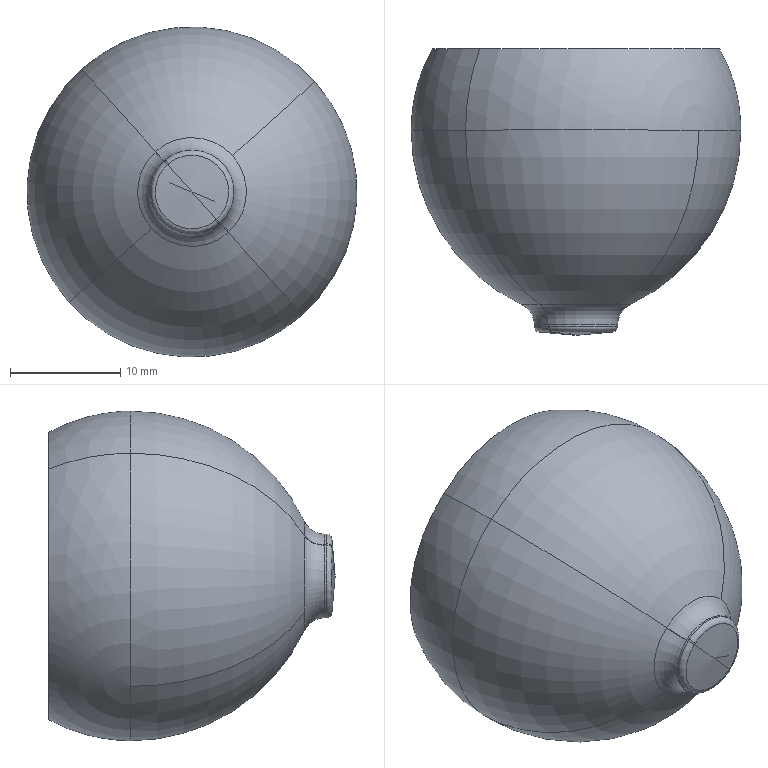Part | SolidWorks | features BaseBody 1 | 1 solid | 44 faces | box 30 x 26.016 x 30 mm | volume 2608 mm3 | torus 20 | cone 12 | sphere 10 | cylinder 2 | commonest cylinder face diameters 7.6 x2
STEP:
#1=CARTESIAN_POINT('',(1944.131,340.517,862.867));
#2=VERTEX_POINT('',#1);
#3=CARTESIAN_POINT('',(1961.977,340.517,843.231));
#4=VERTEX_POINT('',#3);
#5=CARTESIAN_POINT('',(1953.,340.517,853.));
#6=DIRECTION('',(0.,1.,0.));
#7=DIRECTION('',(-0.6685,0.,0.7437));
#8=AXIS2_PLACEMENT_3D('',#5,#6,#7);
#9=CIRCLE('',#8,13.267);
#10=EDGE_CURVE('',#2,#4,#9,.T.);
#11=ORIENTED_EDGE('',*,*,#10,.T.);
#12=CARTESIAN_POINT('',(1961.966,340.482,843.243));
#13=VERTEX_POINT('',#12);
#14=CARTESIAN_POINT('',(1962.094,340.417,843.104));
#15=DIRECTION('',(0.7363,0.,0.6766));
#16=DIRECTION('',(0.6766,0.,-0.7363));
#17=AXIS2_PLACEMENT_3D('',#14,#15,#16);
#18=CIRCLE('',#17,0.2);
#19=EDGE_CURVE('',#4,#13,#18,.T.);
#20=ORIENTED_EDGE('',*,*,#19,.T.);
#21=CARTESIAN_POINT('',(1944.142,340.482,862.855));
#22=VERTEX_POINT('',#21);
#23=CARTESIAN_POINT('',(1953.,340.482,853.));
#24=DIRECTION('',(0.,1.,0.));
#25=DIRECTION('',(-0.6685,0.,0.7437));
#26=AXIS2_PLACEMENT_3D('',#23,#24,#25);
#27=CIRCLE('',#26,13.251);
#28=EDGE_CURVE('',#22,#13,#27,.T.);
#29=ORIENTED_EDGE('',*,*,#28,.F.);
#30=CARTESIAN_POINT('',(1944.016,340.417,862.996));
#31=DIRECTION('',(0.7437,0.,0.6685));
#32=DIRECTION('',(0.5789,0.5,-0.6441));
#33=AXIS2_PLACEMENT_3D('',#30,#31,#32);
#34=CIRCLE('',#33,0.2);
#35=EDGE_CURVE('',#22,#2,#34,.T.);
#36=ORIENTED_EDGE('',*,*,#35,.T.);
#37=EDGE_LOOP('',(#11,#20,#29,#36));
#38=FACE_OUTER_BOUND('',#37,.T.);
#39=CARTESIAN_POINT('',(1953.,340.417,853.));
#40=DIRECTION('',(0.,1.,0.));
#41=DIRECTION('',(0.6766,0.,-0.7363));
#42=AXIS2_PLACEMENT_3D('',#39,#40,#41);
#43=TOROIDAL_SURFACE('',#42,13.44,0.2);
#44=ADVANCED_FACE('',(#38),#43,.T.);
#45=CARTESIAN_POINT('',(1961.869,340.517,843.133));
#46=VERTEX_POINT('',#45);
#47=CARTESIAN_POINT('',(1944.023,340.517,862.769));
#48=VERTEX_POINT('',#47);
#49=CARTESIAN_POINT('',(1953.,340.517,853.));
#50=DIRECTION('',(0.,1.,0.));
#51=DIRECTION('',(0.6685,0.,-0.7437));
#52=AXIS2_PLACEMENT_3D('',#49,#50,#51);
#53=CIRCLE('',#52,13.267);
#54=EDGE_CURVE('',#46,#48,#53,.T.);
#55=ORIENTED_EDGE('',*,*,#54,.T.);
#56=CARTESIAN_POINT('',(1944.034,340.482,862.757));
#57=VERTEX_POINT('',#56);
#58=CARTESIAN_POINT('',(1943.906,340.417,862.896));
#59=DIRECTION('',(-0.7363,0.,-0.6766));
#60=DIRECTION('',(-0.6766,0.,0.7363));
#61=AXIS2_PLACEMENT_3D('',#58,#59,#60);
#62=CIRCLE('',#61,0.2);
#63=EDGE_CURVE('',#48,#57,#62,.T.);
#64=ORIENTED_EDGE('',*,*,#63,.T.);
#65=CARTESIAN_POINT('',(1961.858,340.482,843.145));
#66=VERTEX_POINT('',#65);
#67=CARTESIAN_POINT('',(1953.,340.482,853.));
#68=DIRECTION('',(0.,1.,0.));
#69=DIRECTION('',(0.6685,0.,-0.7437));
#70=AXIS2_PLACEMENT_3D('',#67,#68,#69);
#71=CIRCLE('',#70,13.251);
#72=EDGE_CURVE('',#66,#57,#71,.T.);
#73=ORIENTED_EDGE('',*,*,#72,.F.);
#74=CARTESIAN_POINT('',(1961.984,340.417,843.004));
#75=DIRECTION('',(0.7437,0.,0.6685));
#76=DIRECTION('',(-0.5789,0.5,0.6441));
#77=AXIS2_PLACEMENT_3D('',#74,#75,#76);
#78=CIRCLE('',#77,0.2);
#79=EDGE_CURVE('',#46,#66,#78,.T.);
#80=ORIENTED_EDGE('',*,*,#79,.F.);
#81=EDGE_LOOP('',(#55,#64,#73,#80));
#82=FACE_OUTER_BOUND('',#81,.T.);
#83=CARTESIAN_POINT('',(1953.,340.417,853.));
#84=DIRECTION('',(0.,1.,0.));
#85=DIRECTION('',(-0.6766,0.,0.7363));
#86=AXIS2_PLACEMENT_3D('',#83,#84,#85);
#87=TOROIDAL_SURFACE('',#86,13.44,0.2);
#88=ADVANCED_FACE('',(#82),#87,.T.);
#89=CARTESIAN_POINT('',(1943.95,340.987,863.069));
#90=VERTEX_POINT('',#89);
#91=CARTESIAN_POINT('',(1961.934,340.987,842.828));
#92=VERTEX_POINT('',#91);
#93=CARTESIAN_POINT('',(1953.,340.987,853.));
#94=DIRECTION('',(0.,-1.,0.));
#95=DIRECTION('',(-0.6685,0.,0.7437));
#96=AXIS2_PLACEMENT_3D('',#93,#94,#95);
#97=CIRCLE('',#96,13.538);
#98=EDGE_CURVE('',#90,#92,#97,.T.);
#99=ORIENTED_EDGE('',*,*,#98,.T.);
#100=CARTESIAN_POINT('',(1961.998,341.219,842.755));
#101=VERTEX_POINT('',#100);
#102=CARTESIAN_POINT('',(1961.362,341.487,843.479));
#103=DIRECTION('',(0.7513,0.,0.6599));
#104=DIRECTION('',(0.6599,0.,-0.7513));
#105=AXIS2_PLACEMENT_3D('',#102,#103,#104);
#106=CIRCLE('',#105,1.);
#107=EDGE_CURVE('',#92,#101,#106,.T.);
#108=ORIENTED_EDGE('',*,*,#107,.T.);
#109=CARTESIAN_POINT('',(1943.885,341.219,863.141));
#110=VERTEX_POINT('',#109);
#111=CARTESIAN_POINT('',(1953.,341.219,853.));
#112=DIRECTION('',(0.,-1.,0.));
#113=DIRECTION('',(-0.6685,0.,0.7437));
#114=AXIS2_PLACEMENT_3D('',#111,#112,#113);
#115=CIRCLE('',#114,13.636);
#116=EDGE_CURVE('',#110,#101,#115,.T.);
#117=ORIENTED_EDGE('',*,*,#116,.F.);
#118=CARTESIAN_POINT('',(1944.529,341.487,862.425));
#119=DIRECTION('',(-0.7437,0.,-0.6685));
#120=DIRECTION('',(-0.6442,-0.2672,0.7167));
#121=AXIS2_PLACEMENT_3D('',#118,#119,#120);
#122=CIRCLE('',#121,1.);
#123=EDGE_CURVE('',#90,#110,#122,.T.);
#124=ORIENTED_EDGE('',*,*,#123,.F.);
#125=EDGE_LOOP('',(#99,#108,#117,#124));
#126=FACE_OUTER_BOUND('',#125,.T.);
#127=CARTESIAN_POINT('',(1953.,341.487,853.));
#128=DIRECTION('',(0.,1.,0.));
#129=DIRECTION('',(0.6599,0.,-0.7513));
#130=AXIS2_PLACEMENT_3D('',#127,#128,#129);
#131=TOROIDAL_SURFACE('',#130,12.672,1.);
#132=ADVANCED_FACE('',(#126),#131,.F.);
#133=CARTESIAN_POINT('',(1962.05,340.987,842.931));
#134=VERTEX_POINT('',#133);
#135=CARTESIAN_POINT('',(1944.066,340.987,863.172));
#136=VERTEX_POINT('',#135);
#137=CARTESIAN_POINT('',(1953.,340.987,853.));
#138=DIRECTION('',(0.,-1.,0.));
#139=DIRECTION('',(0.6685,0.,-0.7437));
#140=AXIS2_PLACEMENT_3D('',#137,#138,#139);
#141=CIRCLE('',#140,13.538);
#142=EDGE_CURVE('',#134,#136,#141,.T.);
#143=ORIENTED_EDGE('',*,*,#142,.T.);
#144=CARTESIAN_POINT('',(1944.002,341.219,863.245));
#145=VERTEX_POINT('',#144);
#146=CARTESIAN_POINT('',(1944.638,341.487,862.521));
#147=DIRECTION('',(-0.7513,0.,-0.6599));
#148=DIRECTION('',(-0.6599,0.,0.7513));
#149=AXIS2_PLACEMENT_3D('',#146,#147,#148);
#150=CIRCLE('',#149,1.);
#151=EDGE_CURVE('',#136,#145,#150,.T.);
#152=ORIENTED_EDGE('',*,*,#151,.T.);
#153=CARTESIAN_POINT('',(1962.115,341.219,842.859));
#154=VERTEX_POINT('',#153);
#155=CARTESIAN_POINT('',(1953.,341.219,853.));
#156=DIRECTION('',(0.,-1.,0.));
#157=DIRECTION('',(0.6685,0.,-0.7437));
#158=AXIS2_PLACEMENT_3D('',#155,#156,#157);
#159=CIRCLE('',#158,13.636);
#160=EDGE_CURVE('',#154,#145,#159,.T.);
#161=ORIENTED_EDGE('',*,*,#160,.F.);
#162=CARTESIAN_POINT('',(1961.471,341.487,843.575));
#163=DIRECTION('',(-0.7437,0.,-0.6685));
#164=DIRECTION('',(0.6442,-0.2672,-0.7167));
#165=AXIS2_PLACEMENT_3D('',#162,#163,#164);
#166=CIRCLE('',#165,1.);
#167=EDGE_CURVE('',#154,#134,#166,.T.);
#168=ORIENTED_EDGE('',*,*,#167,.T.);
#169=EDGE_LOOP('',(#143,#152,#161,#168));
#170=FACE_OUTER_BOUND('',#169,.T.);
#171=CARTESIAN_POINT('',(1953.,341.487,853.));
#172=DIRECTION('',(0.,1.,0.));
#173=DIRECTION('',(-0.6599,0.,0.7513));
#174=AXIS2_PLACEMENT_3D('',#171,#172,#173);
#175=TOROIDAL_SURFACE('',#174,12.672,1.);
#176=ADVANCED_FACE('',(#170),#175,.F.);
#177=CARTESIAN_POINT('',(1955.54,327.355,850.174));
#178=VERTEX_POINT('',#177);
#179=CARTESIAN_POINT('',(1950.422,327.355,855.792));
#180=VERTEX_POINT('',#179);
#181=CARTESIAN_POINT('',(1953.,327.355,853.));
#182=DIRECTION('',(0.,1.,0.));
#183=DIRECTION('',(0.6685,0.,-0.7437));
#184=AXIS2_PLACEMENT_3D('',#181,#182,#183);
#185=CIRCLE('',#184,3.8);
#186=EDGE_CURVE('',#178,#180,#185,.T.);
#187=ORIENTED_EDGE('',*,*,#186,.T.);
#188=CARTESIAN_POINT('',(1949.642,329.164,856.636));
#189=VERTEX_POINT('',#188);
#190=CARTESIAN_POINT('',(1949.065,327.355,857.261));
#191=DIRECTION('',(0.7346,0.,0.6785));
#192=DIRECTION('',(0.6785,0.,-0.7346));
#193=AXIS2_PLACEMENT_3D('',#190,#191,#192);
#194=CIRCLE('',#193,2.);
#195=EDGE_CURVE('',#180,#189,#194,.T.);
#196=ORIENTED_EDGE('',*,*,#195,.T.);
#197=CARTESIAN_POINT('',(1949.319,329.164,849.692));
#198=VERTEX_POINT('',#197);
#199=CARTESIAN_POINT('',(1953.,329.164,853.));
#200=DIRECTION('',(0.,1.,0.));
#201=DIRECTION('',(0.6685,0.,-0.7437));
#202=AXIS2_PLACEMENT_3D('',#199,#200,#201);
#203=CIRCLE('',#202,4.949);
#204=EDGE_CURVE('',#198,#189,#203,.T.);
#205=ORIENTED_EDGE('',*,*,#204,.F.);
#206=CARTESIAN_POINT('',(1956.308,329.164,849.319));
#207=VERTEX_POINT('',#206);
#208=CARTESIAN_POINT('',(1953.,329.164,853.));
#209=DIRECTION('',(0.,1.,0.));
#210=DIRECTION('',(0.6685,0.,-0.7437));
#211=AXIS2_PLACEMENT_3D('',#208,#209,#210);
#212=CIRCLE('',#211,4.949);
#213=EDGE_CURVE('',#207,#198,#212,.T.);
#214=ORIENTED_EDGE('',*,*,#213,.F.);
#215=CARTESIAN_POINT('',(1956.877,327.355,848.686));
#216=DIRECTION('',(0.7437,0.,0.6685));
#217=DIRECTION('',(-0.2845,0.9049,0.3166));
#218=AXIS2_PLACEMENT_3D('',#215,#216,#217);
#219=CIRCLE('',#218,2.);
#220=EDGE_CURVE('',#207,#178,#219,.T.);
#221=ORIENTED_EDGE('',*,*,#220,.T.);
#222=EDGE_LOOP('',(#187,#196,#205,#214,#221));
#223=FACE_OUTER_BOUND('',#222,.T.);
#224=CARTESIAN_POINT('',(1953.,327.355,853.));
#225=DIRECTION('',(0.,-1.,0.));
#226=DIRECTION('',(-0.6785,0.,0.7346));
#227=AXIS2_PLACEMENT_3D('',#224,#225,#226);
#228=TOROIDAL_SURFACE('',#227,5.8,2.);
#229=ADVANCED_FACE('',(#223),#228,.F.);
#230=CARTESIAN_POINT('',(1941.844,345.,842.973));
#231=VERTEX_POINT('',#230);
#232=CARTESIAN_POINT('',(1942.973,345.,864.156));
#233=VERTEX_POINT('',#232);
#234=CARTESIAN_POINT('',(1953.,345.,853.));
#235=DIRECTION('',(0.,1.,0.));
#236=DIRECTION('',(0.6685,0.,-0.7437));
#237=AXIS2_PLACEMENT_3D('',#234,#235,#236);
#238=CIRCLE('',#237,15.);
#239=EDGE_CURVE('',#231,#233,#238,.T.);
#240=ORIENTED_EDGE('',*,*,#239,.F.);
#241=CARTESIAN_POINT('',(1954.859,345.,854.671));
#242=DIRECTION('',(-0.6685,0.,0.7437));
#243=DIRECTION('',(0.7437,0.,0.6685));
#244=AXIS2_PLACEMENT_3D('',#241,#242,#243);
#245=CIRCLE('',#244,17.5);
#246=EDGE_CURVE('',#231,#198,#245,.T.);
#247=ORIENTED_EDGE('',*,*,#246,.T.);
#248=ORIENTED_EDGE('',*,*,#204,.T.);
#249=CARTESIAN_POINT('',(1949.692,329.164,856.681));
#250=VERTEX_POINT('',#249);
#251=CARTESIAN_POINT('',(1953.,329.164,853.));
#252=DIRECTION('',(0.,1.,0.));
#253=DIRECTION('',(0.6685,0.,-0.7437));
#254=AXIS2_PLACEMENT_3D('',#251,#252,#253);
#255=CIRCLE('',#254,4.949);
#256=EDGE_CURVE('',#189,#250,#255,.T.);
#257=ORIENTED_EDGE('',*,*,#256,.T.);
#258=CARTESIAN_POINT('',(1954.671,345.,851.141));
#259=DIRECTION('',(0.7437,0.,0.6685));
#260=DIRECTION('',(-0.2845,-0.9049,0.3166));
#261=AXIS2_PLACEMENT_3D('',#258,#259,#260);
#262=CIRCLE('',#261,17.5);
#263=EDGE_CURVE('',#233,#250,#262,.T.);
#264=ORIENTED_EDGE('',*,*,#263,.F.);
#265=EDGE_LOOP('',(#240,#247,#248,#257,#264));
#266=FACE_OUTER_BOUND('',#265,.T.);
#267=CARTESIAN_POINT('',(1953.,345.,853.));
#268=DIRECTION('',(0.,-1.,0.));
#269=DIRECTION('',(0.7437,0.,0.6685));
#270=AXIS2_PLACEMENT_3D('',#267,#268,#269);
#271=TOROIDAL_SURFACE('',#270,-2.5,17.5);
#272=ADVANCED_FACE('',(#266),#271,.T.);
#273=CARTESIAN_POINT('',(1964.156,345.,863.027));
#274=VERTEX_POINT('',#273);
#275=CARTESIAN_POINT('',(1963.027,345.,841.844));
#276=VERTEX_POINT('',#275);
#277=CARTESIAN_POINT('',(1953.,345.,853.));
#278=DIRECTION('',(0.,1.,0.));
#279=DIRECTION('',(-0.6685,0.,0.7437));
#280=AXIS2_PLACEMENT_3D('',#277,#278,#279);
#281=CIRCLE('',#280,15.);
#282=EDGE_CURVE('',#274,#276,#281,.T.);
#283=ORIENTED_EDGE('',*,*,#282,.F.);
#284=CARTESIAN_POINT('',(1956.681,329.164,856.308));
#285=VERTEX_POINT('',#284);
#286=CARTESIAN_POINT('',(1951.141,345.,851.329));
#287=DIRECTION('',(0.6685,0.,-0.7437));
#288=DIRECTION('',(-0.7437,0.,-0.6685));
#289=AXIS2_PLACEMENT_3D('',#286,#287,#288);
#290=CIRCLE('',#289,17.5);
#291=EDGE_CURVE('',#274,#285,#290,.T.);
#292=ORIENTED_EDGE('',*,*,#291,.T.);
#293=CARTESIAN_POINT('',(1956.358,329.164,849.364));
#294=VERTEX_POINT('',#293);
#295=CARTESIAN_POINT('',(1953.,329.164,853.));
#296=DIRECTION('',(0.,1.,0.));
#297=DIRECTION('',(-0.6685,0.,0.7437));
#298=AXIS2_PLACEMENT_3D('',#295,#296,#297);
#299=CIRCLE('',#298,4.949);
#300=EDGE_CURVE('',#285,#294,#299,.T.);
#301=ORIENTED_EDGE('',*,*,#300,.T.);
#302=CARTESIAN_POINT('',(1953.,329.164,853.));
#303=DIRECTION('',(0.,1.,0.));
#304=DIRECTION('',(-0.6685,0.,0.7437));
#305=AXIS2_PLACEMENT_3D('',#302,#303,#304);
#306=CIRCLE('',#305,4.949);
#307=EDGE_CURVE('',#294,#207,#306,.T.);
#308=ORIENTED_EDGE('',*,*,#307,.T.);
#309=CARTESIAN_POINT('',(1951.329,345.,854.859));
#310=DIRECTION('',(0.7437,0.,0.6685));
#311=DIRECTION('',(0.2845,-0.9049,-0.3166));
#312=AXIS2_PLACEMENT_3D('',#309,#310,#311);
#313=CIRCLE('',#312,17.5);
#314=EDGE_CURVE('',#207,#276,#313,.T.);
#315=ORIENTED_EDGE('',*,*,#314,.T.);
#316=EDGE_LOOP('',(#283,#292,#301,#308,#315));
#317=FACE_OUTER_BOUND('',#316,.T.);
#318=CARTESIAN_POINT('',(1953.,345.,853.));
#319=DIRECTION('',(0.,-1.,0.));
#320=DIRECTION('',(0.7437,0.,0.6685));
#321=AXIS2_PLACEMENT_3D('',#318,#319,#320);
#322=TOROIDAL_SURFACE('',#321,-2.5,17.5);
#323=ADVANCED_FACE('',(#317),#322,.T.);
#324=CARTESIAN_POINT('',(1950.46,327.355,855.826));
#325=VERTEX_POINT('',#324);
#326=CARTESIAN_POINT('',(1955.578,327.355,850.208));
#327=VERTEX_POINT('',#326);
#328=CARTESIAN_POINT('',(1953.,327.355,853.));
#329=DIRECTION('',(0.,1.,0.));
#330=DIRECTION('',(-0.6685,0.,0.7437));
#331=AXIS2_PLACEMENT_3D('',#328,#329,#330);
#332=CIRCLE('',#331,3.8);
#333=EDGE_CURVE('',#325,#327,#332,.T.);
#334=ORIENTED_EDGE('',*,*,#333,.T.);
#335=CARTESIAN_POINT('',(1956.935,327.355,848.739));
#336=DIRECTION('',(-0.7346,0.,-0.6785));
#337=DIRECTION('',(-0.6785,0.,0.7346));
#338=AXIS2_PLACEMENT_3D('',#335,#336,#337);
#339=CIRCLE('',#338,2.);
#340=EDGE_CURVE('',#327,#294,#339,.T.);
#341=ORIENTED_EDGE('',*,*,#340,.T.);
#342=ORIENTED_EDGE('',*,*,#300,.F.);
#343=CARTESIAN_POINT('',(1953.,329.164,853.));
#344=DIRECTION('',(0.,1.,0.));
#345=DIRECTION('',(-0.6685,0.,0.7437));
#346=AXIS2_PLACEMENT_3D('',#343,#344,#345);
#347=CIRCLE('',#346,4.949);
#348=EDGE_CURVE('',#250,#285,#347,.T.);
#349=ORIENTED_EDGE('',*,*,#348,.F.);
#350=CARTESIAN_POINT('',(1949.123,327.355,857.314));
#351=DIRECTION('',(0.7437,0.,0.6685));
#352=DIRECTION('',(0.2845,0.9049,-0.3166));
#353=AXIS2_PLACEMENT_3D('',#350,#351,#352);
#354=CIRCLE('',#353,2.);
#355=EDGE_CURVE('',#325,#250,#354,.T.);
#356=ORIENTED_EDGE('',*,*,#355,.F.);
#357=EDGE_LOOP('',(#334,#341,#342,#349,#356));
#358=FACE_OUTER_BOUND('',#357,.T.);
#359=CARTESIAN_POINT('',(1953.,327.355,853.));
#360=DIRECTION('',(0.,-1.,0.));
#361=DIRECTION('',(0.6785,0.,-0.7346));
#362=AXIS2_PLACEMENT_3D('',#359,#360,#361);
#363=TOROIDAL_SURFACE('',#362,5.8,2.);
#364=ADVANCED_FACE('',(#358),#363,.F.);
#365=CARTESIAN_POINT('',(1955.54,327.161,850.174));
#366=VERTEX_POINT('',#365);
#367=CARTESIAN_POINT('',(1950.572,327.161,855.923));
#368=VERTEX_POINT('',#367);
#369=CARTESIAN_POINT('',(1953.,327.161,853.));
#370=DIRECTION('',(0.,-1.,0.));
#371=DIRECTION('',(0.6685,0.,-0.7437));
#372=AXIS2_PLACEMENT_3D('',#369,#370,#371);
#373=CIRCLE('',#372,3.8);
#374=EDGE_CURVE('',#366,#368,#373,.T.);
#375=ORIENTED_EDGE('',*,*,#374,.T.);
#376=CARTESIAN_POINT('',(1950.863,326.663,855.572));
#377=VERTEX_POINT('',#376);
#378=CARTESIAN_POINT('',(1950.891,327.161,855.538));
#379=DIRECTION('',(0.7692,0.,0.639));
#380=DIRECTION('',(0.639,0.,-0.7692));
#381=AXIS2_PLACEMENT_3D('',#378,#379,#380);
#382=CIRCLE('',#381,0.5);
#383=EDGE_CURVE('',#368,#377,#382,.T.);
#384=ORIENTED_EDGE('',*,*,#383,.T.);
#385=CARTESIAN_POINT('',(1955.235,326.663,850.513));
#386=VERTEX_POINT('',#385);
#387=CARTESIAN_POINT('',(1953.,326.663,853.));
#388=DIRECTION('',(0.,-1.,0.));
#389=DIRECTION('',(0.6685,0.,-0.7437));
#390=AXIS2_PLACEMENT_3D('',#387,#388,#389);
#391=CIRCLE('',#390,3.344);
#392=EDGE_CURVE('',#386,#377,#391,.T.);
#393=ORIENTED_EDGE('',*,*,#392,.F.);
#394=CARTESIAN_POINT('',(1955.206,327.161,850.546));
#395=DIRECTION('',(0.7437,0.,0.6685));
#396=DIRECTION('',(0.6685,0.,-0.7437));
#397=AXIS2_PLACEMENT_3D('',#394,#395,#396);
#398=CIRCLE('',#397,0.5);
#399=EDGE_CURVE('',#386,#366,#398,.T.);
#400=ORIENTED_EDGE('',*,*,#399,.T.);
#401=EDGE_LOOP('',(#375,#384,#393,#400));
#402=FACE_OUTER_BOUND('',#401,.T.);
#403=CARTESIAN_POINT('',(1953.,327.161,853.));
#404=DIRECTION('',(0.,-1.,0.));
#405=DIRECTION('',(-0.639,0.,0.7692));
#406=AXIS2_PLACEMENT_3D('',#403,#404,#405);
#407=TOROIDAL_SURFACE('',#406,3.3,0.5);
#408=ADVANCED_FACE('',(#402),#407,.T.);
#409=CARTESIAN_POINT('',(1950.46,327.161,855.826));
#410=VERTEX_POINT('',#409);
#411=CARTESIAN_POINT('',(1955.428,327.161,850.077));
#412=VERTEX_POINT('',#411);
#413=CARTESIAN_POINT('',(1953.,327.161,853.));
#414=DIRECTION('',(0.,-1.,0.));
#415=DIRECTION('',(-0.6685,0.,0.7437));
#416=AXIS2_PLACEMENT_3D('',#413,#414,#415);
#417=CIRCLE('',#416,3.8);
#418=EDGE_CURVE('',#410,#412,#417,.T.);
#419=ORIENTED_EDGE('',*,*,#418,.T.);
#420=CARTESIAN_POINT('',(1955.137,326.663,850.428));
#421=VERTEX_POINT('',#420);
#422=CARTESIAN_POINT('',(1955.109,327.161,850.462));
#423=DIRECTION('',(-0.7692,0.,-0.639));
#424=DIRECTION('',(-0.639,0.,0.7692));
#425=AXIS2_PLACEMENT_3D('',#422,#423,#424);
#426=CIRCLE('',#425,0.5);
#427=EDGE_CURVE('',#412,#421,#426,.T.);
#428=ORIENTED_EDGE('',*,*,#427,.T.);
#429=CARTESIAN_POINT('',(1950.765,326.663,855.487));
#430=VERTEX_POINT('',#429);
#431=CARTESIAN_POINT('',(1953.,326.663,853.));
#432=DIRECTION('',(0.,-1.,0.));
#433=DIRECTION('',(-0.6685,0.,0.7437));
#434=AXIS2_PLACEMENT_3D('',#431,#432,#433);
#435=CIRCLE('',#434,3.344);
#436=EDGE_CURVE('',#430,#421,#435,.T.);
#437=ORIENTED_EDGE('',*,*,#436,.F.);
#438=CARTESIAN_POINT('',(1950.794,327.161,855.454));
#439=DIRECTION('',(0.7437,0.,0.6685));
#440=DIRECTION('',(-0.6685,0.,0.7437));
#441=AXIS2_PLACEMENT_3D('',#438,#439,#440);
#442=CIRCLE('',#441,0.5);
#443=EDGE_CURVE('',#410,#430,#442,.T.);
#444=ORIENTED_EDGE('',*,*,#443,.F.);
#445=EDGE_LOOP('',(#419,#428,#437,#444));
#446=FACE_OUTER_BOUND('',#445,.T.);
#447=CARTESIAN_POINT('',(1953.,327.161,853.));
#448=DIRECTION('',(0.,-1.,0.));
#449=DIRECTION('',(0.639,0.,-0.7692));
#450=AXIS2_PLACEMENT_3D('',#447,#448,#449);
#451=TOROIDAL_SURFACE('',#450,3.3,0.5);
#452=ADVANCED_FACE('',(#446),#451,.T.);
#453=CARTESIAN_POINT('',(1953.,326.37,853.));
#454=VERTEX_POINT('',#453);
#455=CARTESIAN_POINT('',(1953.,326.37,853.));
#456=DIRECTION('',(0.6659,-0.08716,-0.7409));
#457=VECTOR('',#456,1000.);
#458=LINE('',#455,#457);
#459=EDGE_CURVE('',#430,#454,#458,.T.);
#460=ORIENTED_EDGE('',*,*,#459,.F.);
#461=ORIENTED_EDGE('',*,*,#436,.T.);
#462=CARTESIAN_POINT('',(1953.,326.663,853.));
#463=DIRECTION('',(0.,-1.,0.));
#464=DIRECTION('',(-0.6685,0.,0.7437));
#465=AXIS2_PLACEMENT_3D('',#462,#463,#464);
#466=CIRCLE('',#465,3.344);
#467=EDGE_CURVE('',#421,#386,#466,.T.);
#468=ORIENTED_EDGE('',*,*,#467,.T.);
#469=CARTESIAN_POINT('',(1953.,326.37,853.));
#470=DIRECTION('',(0.6659,0.08716,-0.7409));
#471=VECTOR('',#470,1000.);
#472=LINE('',#469,#471);
#473=EDGE_CURVE('',#454,#386,#472,.T.);
#474=ORIENTED_EDGE('',*,*,#473,.F.);
#475=EDGE_LOOP('',(#460,#461,#468,#474));
#476=FACE_OUTER_BOUND('',#475,.T.);
#477=CARTESIAN_POINT('',(1953.,326.521,853.));
#478=DIRECTION('',(0.,1.,0.));
#479=DIRECTION('',(-0.6685,0.,0.7437));
#480=AXIS2_PLACEMENT_3D('',#477,#478,#479);
#481=CONICAL_SURFACE('',#480,1.732,1.484);
#482=ADVANCED_FACE('',(#476),#481,.T.);
#483=ORIENTED_EDGE('',*,*,#427,.F.);
#484=CARTESIAN_POINT('',(1953.,327.161,853.));
#485=DIRECTION('',(0.,-1.,0.));
#486=DIRECTION('',(-0.6685,0.,0.7437));
#487=AXIS2_PLACEMENT_3D('',#484,#485,#486);
#488=CIRCLE('',#487,3.8);
#489=EDGE_CURVE('',#412,#366,#488,.T.);
#490=ORIENTED_EDGE('',*,*,#489,.T.);
#491=ORIENTED_EDGE('',*,*,#399,.F.);
#492=ORIENTED_EDGE('',*,*,#467,.F.);
#493=EDGE_LOOP('',(#483,#490,#491,#492));
#494=FACE_OUTER_BOUND('',#493,.T.);
#495=CARTESIAN_POINT('',(1953.,327.161,853.));
#496=DIRECTION('',(0.,-1.,0.));
#497=DIRECTION('',(0.639,0.,-0.7692));
#498=AXIS2_PLACEMENT_3D('',#495,#496,#497);
#499=TOROIDAL_SURFACE('',#498,3.3,0.5);
#500=ADVANCED_FACE('',(#494),#499,.T.);
#501=CARTESIAN_POINT('',(1955.54,327.161,850.174));
#502=DIRECTION('',(0.,-1.,0.));
#503=VECTOR('',#502,1000.);
#504=LINE('',#501,#503);
#505=EDGE_CURVE('',#178,#366,#504,.T.);
#506=ORIENTED_EDGE('',*,*,#505,.T.);
#507=ORIENTED_EDGE('',*,*,#489,.F.);
#508=ORIENTED_EDGE('',*,*,#418,.F.);
#509=CARTESIAN_POINT('',(1950.46,327.161,855.826));
#510=DIRECTION('',(0.,1.,0.));
#511=VECTOR('',#510,1000.);
#512=LINE('',#509,#511);
#513=EDGE_CURVE('',#410,#325,#512,.T.);
#514=ORIENTED_EDGE('',*,*,#513,.T.);
#515=CARTESIAN_POINT('',(1953.,327.355,853.));
#516=DIRECTION('',(0.,1.,0.));
#517=DIRECTION('',(0.6685,0.,-0.7437));
#518=AXIS2_PLACEMENT_3D('',#515,#516,#517);
#519=CIRCLE('',#518,3.8);
#520=EDGE_CURVE('',#180,#325,#519,.T.);
#521=ORIENTED_EDGE('',*,*,#520,.F.);
#522=ORIENTED_EDGE('',*,*,#186,.F.);
#523=EDGE_LOOP('',(#506,#507,#508,#514,#521,#522));
#524=FACE_OUTER_BOUND('',#523,.T.);
#525=CARTESIAN_POINT('',(1953.,353.807,853.));
#526=DIRECTION('',(0.,-1.,0.));
#527=DIRECTION('',(0.6685,0.,-0.7437));
#528=AXIS2_PLACEMENT_3D('',#525,#526,#527);
#529=CYLINDRICAL_SURFACE('',#528,3.8);
#530=ADVANCED_FACE('',(#524),#529,.T.);
#531=ORIENTED_EDGE('',*,*,#513,.F.);
#532=CARTESIAN_POINT('',(1953.,327.161,853.));
#533=DIRECTION('',(0.,-1.,0.));
#534=DIRECTION('',(0.6685,0.,-0.7437));
#535=AXIS2_PLACEMENT_3D('',#532,#533,#534);
#536=CIRCLE('',#535,3.8);
#537=EDGE_CURVE('',#368,#410,#536,.T.);
#538=ORIENTED_EDGE('',*,*,#537,.F.);
#539=ORIENTED_EDGE('',*,*,#374,.F.);
#540=ORIENTED_EDGE('',*,*,#505,.F.);
#541=CARTESIAN_POINT('',(1953.,327.355,853.));
#542=DIRECTION('',(0.,1.,0.));
#543=DIRECTION('',(-0.6685,0.,0.7437));
#544=AXIS2_PLACEMENT_3D('',#541,#542,#543);
#545=CIRCLE('',#544,3.8);
#546=EDGE_CURVE('',#327,#178,#545,.T.);
#547=ORIENTED_EDGE('',*,*,#546,.F.);
#548=ORIENTED_EDGE('',*,*,#333,.F.);
#549=EDGE_LOOP('',(#531,#538,#539,#540,#547,#548));
#550=FACE_OUTER_BOUND('',#549,.T.);
#551=CARTESIAN_POINT('',(1953.,353.807,853.));
#552=DIRECTION('',(0.,-1.,0.));
#553=DIRECTION('',(0.6685,0.,-0.7437));
#554=AXIS2_PLACEMENT_3D('',#551,#552,#553);
#555=CYLINDRICAL_SURFACE('',#554,3.8);
#556=ADVANCED_FACE('',(#550),#555,.T.);
#557=ORIENTED_EDGE('',*,*,#383,.F.);
#558=ORIENTED_EDGE('',*,*,#537,.T.);
#559=ORIENTED_EDGE('',*,*,#443,.T.);
#560=CARTESIAN_POINT('',(1953.,326.663,853.));
#561=DIRECTION('',(0.,-1.,0.));
#562=DIRECTION('',(0.6685,0.,-0.7437));
#563=AXIS2_PLACEMENT_3D('',#560,#561,#562);
#564=CIRCLE('',#563,3.344);
#565=EDGE_CURVE('',#377,#430,#564,.T.);
#566=ORIENTED_EDGE('',*,*,#565,.F.);
#567=EDGE_LOOP('',(#557,#558,#559,#566));
#568=FACE_OUTER_BOUND('',#567,.T.);
#569=CARTESIAN_POINT('',(1953.,327.161,853.));
#570=DIRECTION('',(0.,-1.,0.));
#571=DIRECTION('',(-0.639,0.,0.7692));
#572=AXIS2_PLACEMENT_3D('',#569,#570,#571);
#573=TOROIDAL_SURFACE('',#572,3.3,0.5);
#574=ADVANCED_FACE('',(#568),#573,.T.);
#575=ORIENTED_EDGE('',*,*,#473,.T.);
#576=ORIENTED_EDGE('',*,*,#392,.T.);
#577=ORIENTED_EDGE('',*,*,#565,.T.);
#578=ORIENTED_EDGE('',*,*,#459,.T.);
#579=EDGE_LOOP('',(#575,#576,#577,#578));
#580=FACE_OUTER_BOUND('',#579,.T.);
#581=CARTESIAN_POINT('',(1953.,326.521,853.));
#582=DIRECTION('',(0.,1.,0.));
#583=DIRECTION('',(-0.6685,0.,0.7437));
#584=AXIS2_PLACEMENT_3D('',#581,#582,#583);
#585=CONICAL_SURFACE('',#584,1.732,1.484);
#586=ADVANCED_FACE('',(#580),#585,.T.);
#587=ORIENTED_EDGE('',*,*,#340,.F.);
#588=ORIENTED_EDGE('',*,*,#546,.T.);
#589=ORIENTED_EDGE('',*,*,#220,.F.);
#590=ORIENTED_EDGE('',*,*,#307,.F.);
#591=EDGE_LOOP('',(#587,#588,#589,#590));
#592=FACE_OUTER_BOUND('',#591,.T.);
#593=CARTESIAN_POINT('',(1953.,327.355,853.));
#594=DIRECTION('',(0.,-1.,0.));
#595=DIRECTION('',(0.6785,0.,-0.7346));
#596=AXIS2_PLACEMENT_3D('',#593,#594,#595);
#597=TOROIDAL_SURFACE('',#596,5.8,2.);
#598=ADVANCED_FACE('',(#592),#597,.F.);
#599=ORIENTED_EDGE('',*,*,#291,.F.);
#600=CARTESIAN_POINT('',(1953.,345.,853.));
#601=DIRECTION('',(0.,1.,0.));
#602=DIRECTION('',(-0.6685,0.,0.7437));
#603=AXIS2_PLACEMENT_3D('',#600,#601,#602);
#604=CIRCLE('',#603,15.);
#605=EDGE_CURVE('',#233,#274,#604,.T.);
#606=ORIENTED_EDGE('',*,*,#605,.F.);
#607=ORIENTED_EDGE('',*,*,#263,.T.);
#608=ORIENTED_EDGE('',*,*,#348,.T.);
#609=EDGE_LOOP('',(#599,#606,#607,#608));
#610=FACE_OUTER_BOUND('',#609,.T.);
#611=CARTESIAN_POINT('',(1953.,345.,853.));
#612=DIRECTION('',(0.,-1.,0.));
#613=DIRECTION('',(0.7437,0.,0.6685));
#614=AXIS2_PLACEMENT_3D('',#611,#612,#613);
#615=TOROIDAL_SURFACE('',#614,-2.5,17.5);
#616=ADVANCED_FACE('',(#610),#615,.T.);
#617=CARTESIAN_POINT('',(1944.273,352.386,862.71));
#618=VERTEX_POINT('',#617);
#619=CARTESIAN_POINT('',(1953.,345.,853.));
#620=DIRECTION('',(0.7437,0.,0.6685));
#621=DIRECTION('',(-0.6685,0.,0.7437));
#622=AXIS2_PLACEMENT_3D('',#619,#620,#621);
#623=CIRCLE('',#622,15.);
#624=EDGE_CURVE('',#618,#233,#623,.T.);
#625=ORIENTED_EDGE('',*,*,#624,.T.);
#626=ORIENTED_EDGE('',*,*,#605,.T.);
#627=ORIENTED_EDGE('',*,*,#282,.T.);
#628=CARTESIAN_POINT('',(1961.727,352.386,843.29));
#629=VERTEX_POINT('',#628);
#630=CARTESIAN_POINT('',(1953.,345.,853.));
#631=DIRECTION('',(0.7437,0.,0.6685));
#632=DIRECTION('',(0.6685,0.,-0.7437));
#633=AXIS2_PLACEMENT_3D('',#630,#631,#632);
#634=CIRCLE('',#633,15.);
#635=EDGE_CURVE('',#276,#629,#634,.T.);
#636=ORIENTED_EDGE('',*,*,#635,.T.);
#637=CARTESIAN_POINT('',(1953.,352.386,853.));
#638=DIRECTION('',(0.,-1.,0.));
#639=DIRECTION('',(0.6685,0.,-0.7437));
#640=AXIS2_PLACEMENT_3D('',#637,#638,#639);
#641=CIRCLE('',#640,13.055);
#642=EDGE_CURVE('',#629,#618,#641,.T.);
#643=ORIENTED_EDGE('',*,*,#642,.T.);
#644=EDGE_LOOP('',(#625,#626,#627,#636,#643));
#645=FACE_OUTER_BOUND('',#644,.T.);
#646=CARTESIAN_POINT('',(1953.,345.,853.));
#647=DIRECTION('',(0.7437,0.,0.6685));
#648=DIRECTION('',(0.6685,0.,-0.7437));
#649=AXIS2_PLACEMENT_3D('',#646,#647,#648);
#650=SPHERICAL_SURFACE('',#649,15.);
#651=ADVANCED_FACE('',(#645),#650,.T.);
#652=ORIENTED_EDGE('',*,*,#635,.F.);
#653=CARTESIAN_POINT('',(1953.,345.,853.));
#654=DIRECTION('',(0.,1.,0.));
#655=DIRECTION('',(0.6685,0.,-0.7437));
#656=AXIS2_PLACEMENT_3D('',#653,#654,#655);
#657=CIRCLE('',#656,15.);
#658=EDGE_CURVE('',#276,#231,#657,.T.);
#659=ORIENTED_EDGE('',*,*,#658,.T.);
#660=ORIENTED_EDGE('',*,*,#239,.T.);
#661=ORIENTED_EDGE('',*,*,#624,.F.);
#662=CARTESIAN_POINT('',(1953.,352.386,853.));
#663=DIRECTION('',(0.,1.,0.));
#664=DIRECTION('',(0.6685,0.,-0.7437));
#665=AXIS2_PLACEMENT_3D('',#662,#663,#664);
#666=CIRCLE('',#665,13.055);
#667=EDGE_CURVE('',#629,#618,#666,.T.);
#668=ORIENTED_EDGE('',*,*,#667,.F.);
#669=EDGE_LOOP('',(#652,#659,#660,#661,#668));
#670=FACE_OUTER_BOUND('',#669,.T.);
#671=CARTESIAN_POINT('',(1953.,345.,853.));
#672=DIRECTION('',(0.7437,0.,0.6685));
#673=DIRECTION('',(0.6685,0.,-0.7437));
#674=AXIS2_PLACEMENT_3D('',#671,#672,#673);
#675=SPHERICAL_SURFACE('',#674,15.);
#676=ADVANCED_FACE('',(#670),#675,.T.);
#677=ORIENTED_EDGE('',*,*,#246,.F.);
#678=ORIENTED_EDGE('',*,*,#658,.F.);
#679=ORIENTED_EDGE('',*,*,#314,.F.);
#680=ORIENTED_EDGE('',*,*,#213,.T.);
#681=EDGE_LOOP('',(#677,#678,#679,#680));
#682=FACE_OUTER_BOUND('',#681,.T.);
#683=CARTESIAN_POINT('',(1953.,345.,853.));
#684=DIRECTION('',(0.,-1.,0.));
#685=DIRECTION('',(0.7437,0.,0.6685));
#686=AXIS2_PLACEMENT_3D('',#683,#684,#685);
#687=TOROIDAL_SURFACE('',#686,-2.5,17.5);
#688=ADVANCED_FACE('',(#682),#687,.T.);
#689=ORIENTED_EDGE('',*,*,#195,.F.);
#690=ORIENTED_EDGE('',*,*,#520,.T.);
#691=ORIENTED_EDGE('',*,*,#355,.T.);
#692=ORIENTED_EDGE('',*,*,#256,.F.);
#693=EDGE_LOOP('',(#689,#690,#691,#692));
#694=FACE_OUTER_BOUND('',#693,.T.);
#695=CARTESIAN_POINT('',(1953.,327.355,853.));
#696=DIRECTION('',(0.,-1.,0.));
#697=DIRECTION('',(-0.6785,0.,0.7346));
#698=AXIS2_PLACEMENT_3D('',#695,#696,#697);
#699=TOROIDAL_SURFACE('',#698,5.8,2.);
#700=ADVANCED_FACE('',(#694),#699,.F.);
#701=CARTESIAN_POINT('',(1944.622,352.091,862.321));
#702=VERTEX_POINT('',#701);
#703=CARTESIAN_POINT('',(1944.622,352.091,862.321));
#704=DIRECTION('',(-0.5818,0.4924,0.6473));
#705=VECTOR('',#704,1000.);
#706=LINE('',#703,#705);
#707=EDGE_CURVE('',#702,#618,#706,.T.);
#708=ORIENTED_EDGE('',*,*,#707,.F.);
#709=CARTESIAN_POINT('',(1961.378,352.091,843.679));
#710=VERTEX_POINT('',#709);
#711=CARTESIAN_POINT('',(1953.,352.091,853.));
#712=DIRECTION('',(0.,1.,0.));
#713=DIRECTION('',(0.6685,0.,-0.7437));
#714=AXIS2_PLACEMENT_3D('',#711,#712,#713);
#715=CIRCLE('',#714,12.533);
#716=EDGE_CURVE('',#710,#702,#715,.T.);
#717=ORIENTED_EDGE('',*,*,#716,.F.);
#718=CARTESIAN_POINT('',(1961.727,352.386,843.29));
#719=DIRECTION('',(-0.5818,-0.4924,0.6473));
#720=VECTOR('',#719,1000.);
#721=LINE('',#718,#720);
#722=EDGE_CURVE('',#629,#710,#721,.T.);
#723=ORIENTED_EDGE('',*,*,#722,.F.);
#724=ORIENTED_EDGE('',*,*,#667,.T.);
#725=EDGE_LOOP('',(#708,#717,#723,#724));
#726=FACE_OUTER_BOUND('',#725,.T.);
#727=CARTESIAN_POINT('',(1953.,352.239,853.));
#728=DIRECTION('',(0.,1.,0.));
#729=DIRECTION('',(-0.6685,0.,0.7437));
#730=AXIS2_PLACEMENT_3D('',#727,#728,#729);
#731=CONICAL_SURFACE('',#730,12.794,1.056);
#732=ADVANCED_FACE('',(#726),#731,.F.);
#733=CARTESIAN_POINT('',(1961.276,351.538,843.793));
#734=VERTEX_POINT('',#733);
#735=CARTESIAN_POINT('',(1961.276,351.538,843.793));
#736=DIRECTION('',(-0.1786,-0.9636,0.1988));
#737=VECTOR('',#736,1000.);
#738=LINE('',#735,#737);
#739=EDGE_CURVE('',#710,#734,#738,.T.);
#740=ORIENTED_EDGE('',*,*,#739,.F.);
#741=ORIENTED_EDGE('',*,*,#716,.T.);
#742=CARTESIAN_POINT('',(1944.724,351.538,862.207));
#743=VERTEX_POINT('',#742);
#744=CARTESIAN_POINT('',(1944.724,351.538,862.207));
#745=DIRECTION('',(-0.1786,0.9636,0.1988));
#746=VECTOR('',#745,1000.);
#747=LINE('',#744,#746);
#748=EDGE_CURVE('',#743,#702,#747,.T.);
#749=ORIENTED_EDGE('',*,*,#748,.F.);
#750=CARTESIAN_POINT('',(1953.,351.538,853.));
#751=DIRECTION('',(0.,-1.,0.));
#752=DIRECTION('',(-0.6685,0.,0.7437));
#753=AXIS2_PLACEMENT_3D('',#750,#751,#752);
#754=CIRCLE('',#753,12.38);
#755=EDGE_CURVE('',#743,#734,#754,.T.);
#756=ORIENTED_EDGE('',*,*,#755,.T.);
#757=EDGE_LOOP('',(#740,#741,#749,#756));
#758=FACE_OUTER_BOUND('',#757,.T.);
#759=CARTESIAN_POINT('',(1953.,351.814,853.));
#760=DIRECTION('',(0.,1.,0.));
#761=DIRECTION('',(-0.6685,0.,0.7437));
#762=AXIS2_PLACEMENT_3D('',#759,#760,#761);
#763=CONICAL_SURFACE('',#762,12.456,0.2705);
#764=ADVANCED_FACE('',(#758),#763,.F.);
#765=ORIENTED_EDGE('',*,*,#748,.T.);
#766=CARTESIAN_POINT('',(1953.,352.091,853.));
#767=DIRECTION('',(0.,1.,0.));
#768=DIRECTION('',(-0.6685,0.,0.7437));
#769=AXIS2_PLACEMENT_3D('',#766,#767,#768);
#770=CIRCLE('',#769,12.533);
#771=EDGE_CURVE('',#702,#710,#770,.T.);
#772=ORIENTED_EDGE('',*,*,#771,.T.);
#773=ORIENTED_EDGE('',*,*,#739,.T.);
#774=CARTESIAN_POINT('',(1953.,351.538,853.));
#775=DIRECTION('',(0.,-1.,0.));
#776=DIRECTION('',(0.6685,0.,-0.7437));
#777=AXIS2_PLACEMENT_3D('',#774,#775,#776);
#778=CIRCLE('',#777,12.38);
#779=EDGE_CURVE('',#734,#743,#778,.T.);
#780=ORIENTED_EDGE('',*,*,#779,.T.);
#781=EDGE_LOOP('',(#765,#772,#773,#780));
#782=FACE_OUTER_BOUND('',#781,.T.);
#783=CARTESIAN_POINT('',(1953.,351.814,853.));
#784=DIRECTION('',(0.,1.,0.));
#785=DIRECTION('',(-0.6685,0.,0.7437));
#786=AXIS2_PLACEMENT_3D('',#783,#784,#785);
#787=CONICAL_SURFACE('',#786,12.456,0.2705);
#788=ADVANCED_FACE('',(#782),#787,.F.);
#789=ORIENTED_EDGE('',*,*,#722,.T.);
#790=ORIENTED_EDGE('',*,*,#771,.F.);
#791=ORIENTED_EDGE('',*,*,#707,.T.);
#792=ORIENTED_EDGE('',*,*,#642,.F.);
#793=EDGE_LOOP('',(#789,#790,#791,#792));
#794=FACE_OUTER_BOUND('',#793,.T.);
#795=CARTESIAN_POINT('',(1953.,352.239,853.));
#796=DIRECTION('',(0.,1.,0.));
#797=DIRECTION('',(-0.6685,0.,0.7437));
#798=AXIS2_PLACEMENT_3D('',#795,#796,#797);
#799=CONICAL_SURFACE('',#798,12.794,1.056);
#800=ADVANCED_FACE('',(#794),#799,.F.);
#801=CARTESIAN_POINT('',(1944.106,349.355,862.896));
#802=VERTEX_POINT('',#801);
#803=CARTESIAN_POINT('',(1953.,345.,853.));
#804=DIRECTION('',(-0.7437,0.,-0.6685));
#805=DIRECTION('',(-0.6353,0.3111,0.7068));
#806=AXIS2_PLACEMENT_3D('',#803,#804,#805);
#807=CIRCLE('',#806,14.);
#808=EDGE_CURVE('',#802,#743,#807,.T.);
#809=ORIENTED_EDGE('',*,*,#808,.T.);
#810=ORIENTED_EDGE('',*,*,#779,.F.);
#811=CARTESIAN_POINT('',(1961.894,349.355,843.104));
#812=VERTEX_POINT('',#811);
#813=CARTESIAN_POINT('',(1953.,345.,853.));
#814=DIRECTION('',(-0.7437,0.,-0.6685));
#815=DIRECTION('',(0.5911,0.467,-0.6577));
#816=AXIS2_PLACEMENT_3D('',#813,#814,#815);
#817=CIRCLE('',#816,14.);
#818=EDGE_CURVE('',#734,#812,#817,.T.);
#819=ORIENTED_EDGE('',*,*,#818,.T.);
#820=CARTESIAN_POINT('',(1953.,349.355,853.));
#821=DIRECTION('',(0.,-1.,0.));
#822=DIRECTION('',(0.6685,0.,-0.7437));
#823=AXIS2_PLACEMENT_3D('',#820,#821,#822);
#824=CIRCLE('',#823,13.305);
#825=EDGE_CURVE('',#812,#802,#824,.T.);
#826=ORIENTED_EDGE('',*,*,#825,.T.);
#827=EDGE_LOOP('',(#809,#810,#819,#826));
#828=FACE_OUTER_BOUND('',#827,.T.);
#829=CARTESIAN_POINT('',(1953.,345.,853.));
#830=DIRECTION('',(0.7437,0.,0.6685));
#831=DIRECTION('',(0.6685,0.,-0.7437));
#832=AXIS2_PLACEMENT_3D('',#829,#830,#831);
#833=SPHERICAL_SURFACE('',#832,14.);
#834=ADVANCED_FACE('',(#828),#833,.F.);
#835=ORIENTED_EDGE('',*,*,#818,.F.);
#836=ORIENTED_EDGE('',*,*,#755,.F.);
#837=ORIENTED_EDGE('',*,*,#808,.F.);
#838=CARTESIAN_POINT('',(1953.,349.355,853.));
#839=DIRECTION('',(0.,1.,0.));
#840=DIRECTION('',(0.6685,0.,-0.7437));
#841=AXIS2_PLACEMENT_3D('',#838,#839,#840);
#842=CIRCLE('',#841,13.305);
#843=EDGE_CURVE('',#812,#802,#842,.T.);
#844=ORIENTED_EDGE('',*,*,#843,.F.);
#845=EDGE_LOOP('',(#835,#836,#837,#844));
#846=FACE_OUTER_BOUND('',#845,.T.);
#847=CARTESIAN_POINT('',(1953.,345.,853.));
#848=DIRECTION('',(0.7437,0.,0.6685));
#849=DIRECTION('',(0.6685,0.,-0.7437));
#850=AXIS2_PLACEMENT_3D('',#847,#848,#849);
#851=SPHERICAL_SURFACE('',#850,14.);
#852=ADVANCED_FACE('',(#846),#851,.F.);
#853=CARTESIAN_POINT('',(1943.977,349.248,863.039));
#854=VERTEX_POINT('',#853);
#855=CARTESIAN_POINT('',(1944.106,349.355,862.896));
#856=DIRECTION('',(-0.583,-0.4894,0.6486));
#857=VECTOR('',#856,1000.);
#858=LINE('',#855,#857);
#859=EDGE_CURVE('',#802,#854,#858,.T.);
#860=ORIENTED_EDGE('',*,*,#859,.T.);
#861=CARTESIAN_POINT('',(1962.023,349.248,842.961));
#862=VERTEX_POINT('',#861);
#863=CARTESIAN_POINT('',(1953.,349.248,853.));
#864=DIRECTION('',(0.,1.,0.));
#865=DIRECTION('',(0.6685,0.,-0.7437));
#866=AXIS2_PLACEMENT_3D('',#863,#864,#865);
#867=CIRCLE('',#866,13.497);
#868=EDGE_CURVE('',#862,#854,#867,.T.);
#869=ORIENTED_EDGE('',*,*,#868,.F.);
#870=CARTESIAN_POINT('',(1961.894,349.355,843.104));
#871=DIRECTION('',(-0.583,0.4894,0.6486));
#872=VECTOR('',#871,1000.);
#873=LINE('',#870,#872);
#874=EDGE_CURVE('',#862,#812,#873,.T.);
#875=ORIENTED_EDGE('',*,*,#874,.T.);
#876=ORIENTED_EDGE('',*,*,#843,.T.);
#877=EDGE_LOOP('',(#860,#869,#875,#876));
#878=FACE_OUTER_BOUND('',#877,.T.);
#879=CARTESIAN_POINT('',(1953.,349.302,853.));
#880=DIRECTION('',(0.,-1.,0.));
#881=DIRECTION('',(0.6685,0.,-0.7437));
#882=AXIS2_PLACEMENT_3D('',#879,#880,#881);
#883=CONICAL_SURFACE('',#882,13.401,1.059);
#884=ADVANCED_FACE('',(#878),#883,.F.);
#885=CARTESIAN_POINT('',(1953.,345.,853.));
#886=DIRECTION('',(-0.7437,0.,-0.6685));
#887=DIRECTION('',(0.6376,0.3002,-0.7094));
#888=AXIS2_PLACEMENT_3D('',#885,#886,#887);
#889=CIRCLE('',#888,14.15);
#890=EDGE_CURVE('',#862,#154,#889,.T.);
#891=ORIENTED_EDGE('',*,*,#890,.F.);
#892=ORIENTED_EDGE('',*,*,#868,.T.);
#893=CARTESIAN_POINT('',(1953.,345.,853.));
#894=DIRECTION('',(-0.7437,0.,-0.6685));
#895=DIRECTION('',(-0.6442,-0.2672,0.7167));
#896=AXIS2_PLACEMENT_3D('',#893,#894,#895);
#897=CIRCLE('',#896,14.15);
#898=EDGE_CURVE('',#110,#854,#897,.T.);
#899=ORIENTED_EDGE('',*,*,#898,.F.);
#900=ORIENTED_EDGE('',*,*,#116,.T.);
#901=CARTESIAN_POINT('',(1953.,341.219,853.));
#902=DIRECTION('',(0.,-1.,0.));
#903=DIRECTION('',(-0.6685,0.,0.7437));
#904=AXIS2_PLACEMENT_3D('',#901,#902,#903);
#905=CIRCLE('',#904,13.636);
#906=EDGE_CURVE('',#101,#154,#905,.T.);
#907=ORIENTED_EDGE('',*,*,#906,.T.);
#908=EDGE_LOOP('',(#891,#892,#899,#900,#907));
#909=FACE_OUTER_BOUND('',#908,.T.);
#910=CARTESIAN_POINT('',(1953.,345.,853.));
#911=DIRECTION('',(0.7437,0.,0.6685));
#912=DIRECTION('',(-0.6685,0.,0.7437));
#913=AXIS2_PLACEMENT_3D('',#910,#911,#912);
#914=SPHERICAL_SURFACE('',#913,14.15);
#915=ADVANCED_FACE('',(#909),#914,.F.);
#916=ORIENTED_EDGE('',*,*,#898,.T.);
#917=CARTESIAN_POINT('',(1953.,349.248,853.));
#918=DIRECTION('',(0.,1.,0.));
#919=DIRECTION('',(-0.6685,0.,0.7437));
#920=AXIS2_PLACEMENT_3D('',#917,#918,#919);
#921=CIRCLE('',#920,13.497);
#922=EDGE_CURVE('',#854,#862,#921,.T.);
#923=ORIENTED_EDGE('',*,*,#922,.T.);
#924=ORIENTED_EDGE('',*,*,#890,.T.);
#925=ORIENTED_EDGE('',*,*,#160,.T.);
#926=CARTESIAN_POINT('',(1953.,341.219,853.));
#927=DIRECTION('',(0.,-1.,0.));
#928=DIRECTION('',(0.6685,0.,-0.7437));
#929=AXIS2_PLACEMENT_3D('',#926,#927,#928);
#930=CIRCLE('',#929,13.636);
#931=EDGE_CURVE('',#145,#110,#930,.T.);
#932=ORIENTED_EDGE('',*,*,#931,.T.);
#933=EDGE_LOOP('',(#916,#923,#924,#925,#932));
#934=FACE_OUTER_BOUND('',#933,.T.);
#935=CARTESIAN_POINT('',(1953.,345.,853.));
#936=DIRECTION('',(0.7437,0.,0.6685));
#937=DIRECTION('',(-0.6685,0.,0.7437));
#938=AXIS2_PLACEMENT_3D('',#935,#936,#937);
#939=SPHERICAL_SURFACE('',#938,14.15);
#940=ADVANCED_FACE('',(#934),#939,.F.);
#941=ORIENTED_EDGE('',*,*,#874,.F.);
#942=ORIENTED_EDGE('',*,*,#922,.F.);
#943=ORIENTED_EDGE('',*,*,#859,.F.);
#944=ORIENTED_EDGE('',*,*,#825,.F.);
#945=EDGE_LOOP('',(#941,#942,#943,#944));
#946=FACE_OUTER_BOUND('',#945,.T.);
#947=CARTESIAN_POINT('',(1953.,349.302,853.));
#948=DIRECTION('',(0.,-1.,0.));
#949=DIRECTION('',(0.6685,0.,-0.7437));
#950=AXIS2_PLACEMENT_3D('',#947,#948,#949);
#951=CONICAL_SURFACE('',#950,13.401,1.059);
#952=ADVANCED_FACE('',(#946),#951,.F.);
#953=ORIENTED_EDGE('',*,*,#151,.F.);
#954=CARTESIAN_POINT('',(1953.,340.987,853.));
#955=DIRECTION('',(0.,-1.,0.));
#956=DIRECTION('',(0.6685,0.,-0.7437));
#957=AXIS2_PLACEMENT_3D('',#954,#955,#956);
#958=CIRCLE('',#957,13.538);
#959=EDGE_CURVE('',#136,#90,#958,.T.);
#960=ORIENTED_EDGE('',*,*,#959,.T.);
#961=ORIENTED_EDGE('',*,*,#123,.T.);
#962=ORIENTED_EDGE('',*,*,#931,.F.);
#963=EDGE_LOOP('',(#953,#960,#961,#962));
#964=FACE_OUTER_BOUND('',#963,.T.);
#965=CARTESIAN_POINT('',(1953.,341.487,853.));
#966=DIRECTION('',(0.,1.,0.));
#967=DIRECTION('',(-0.6599,0.,0.7513));
#968=AXIS2_PLACEMENT_3D('',#965,#966,#967);
#969=TOROIDAL_SURFACE('',#968,12.672,1.);
#970=ADVANCED_FACE('',(#964),#969,.F.);
#971=ORIENTED_EDGE('',*,*,#107,.F.);
#972=CARTESIAN_POINT('',(1953.,340.987,853.));
#973=DIRECTION('',(0.,-1.,0.));
#974=DIRECTION('',(-0.6685,0.,0.7437));
#975=AXIS2_PLACEMENT_3D('',#972,#973,#974);
#976=CIRCLE('',#975,13.538);
#977=EDGE_CURVE('',#92,#134,#976,.T.);
#978=ORIENTED_EDGE('',*,*,#977,.T.);
#979=ORIENTED_EDGE('',*,*,#167,.F.);
#980=ORIENTED_EDGE('',*,*,#906,.F.);
#981=EDGE_LOOP('',(#971,#978,#979,#980));
#982=FACE_OUTER_BOUND('',#981,.T.);
#983=CARTESIAN_POINT('',(1953.,341.487,853.));
#984=DIRECTION('',(0.,1.,0.));
#985=DIRECTION('',(0.6599,0.,-0.7513));
#986=AXIS2_PLACEMENT_3D('',#983,#984,#985);
#987=TOROIDAL_SURFACE('',#986,12.672,1.);
#988=ADVANCED_FACE('',(#982),#987,.F.);
#989=CARTESIAN_POINT('',(1944.131,340.517,862.867));
#990=DIRECTION('',(0.3342,-0.866,-0.3719));
#991=VECTOR('',#990,1000.);
#992=LINE('',#989,#991);
#993=EDGE_CURVE('',#90,#2,#992,.T.);
#994=ORIENTED_EDGE('',*,*,#993,.T.);
#995=CARTESIAN_POINT('',(1953.,340.517,853.));
#996=DIRECTION('',(0.,1.,0.));
#997=DIRECTION('',(0.6685,0.,-0.7437));
#998=AXIS2_PLACEMENT_3D('',#995,#996,#997);
#999=CIRCLE('',#998,13.267);
#1000=EDGE_CURVE('',#48,#2,#999,.T.);
#1001=ORIENTED_EDGE('',*,*,#1000,.F.);
#1002=ORIENTED_EDGE('',*,*,#54,.F.);
#1003=CARTESIAN_POINT('',(1961.869,340.517,843.133));
#1004=DIRECTION('',(0.3342,0.866,-0.3719));
#1005=VECTOR('',#1004,1000.);
#1006=LINE('',#1003,#1005);
#1007=EDGE_CURVE('',#46,#134,#1006,.T.);
#1008=ORIENTED_EDGE('',*,*,#1007,.T.);
#1009=ORIENTED_EDGE('',*,*,#977,.F.);
#1010=ORIENTED_EDGE('',*,*,#98,.F.);
#1011=EDGE_LOOP('',(#994,#1001,#1002,#1008,#1009,#1010));
#1012=FACE_OUTER_BOUND('',#1011,.T.);
#1013=CARTESIAN_POINT('',(1953.,340.752,853.));
#1014=DIRECTION('',(0.,1.,0.));
#1015=DIRECTION('',(-0.6685,0.,0.7437));
#1016=AXIS2_PLACEMENT_3D('',#1013,#1014,#1015);
#1017=CONICAL_SURFACE('',#1016,13.402,0.5236);
#1018=ADVANCED_FACE('',(#1012),#1017,.F.);
#1019=ORIENTED_EDGE('',*,*,#63,.F.);
#1020=ORIENTED_EDGE('',*,*,#1000,.T.);
#1021=ORIENTED_EDGE('',*,*,#35,.F.);
#1022=CARTESIAN_POINT('',(1953.,340.482,853.));
#1023=DIRECTION('',(0.,1.,0.));
#1024=DIRECTION('',(0.6685,0.,-0.7437));
#1025=AXIS2_PLACEMENT_3D('',#1022,#1023,#1024);
#1026=CIRCLE('',#1025,13.251);
#1027=EDGE_CURVE('',#57,#22,#1026,.T.);
#1028=ORIENTED_EDGE('',*,*,#1027,.F.);
#1029=EDGE_LOOP('',(#1019,#1020,#1021,#1028));
#1030=FACE_OUTER_BOUND('',#1029,.T.);
#1031=CARTESIAN_POINT('',(1953.,340.417,853.));
#1032=DIRECTION('',(0.,1.,0.));
#1033=DIRECTION('',(-0.6766,0.,0.7363));
#1034=AXIS2_PLACEMENT_3D('',#1031,#1032,#1033);
#1035=TOROIDAL_SURFACE('',#1034,13.44,0.2);
#1036=ADVANCED_FACE('',(#1030),#1035,.T.);
#1037=ORIENTED_EDGE('',*,*,#19,.F.);
#1038=CARTESIAN_POINT('',(1953.,340.517,853.));
#1039=DIRECTION('',(0.,1.,0.));
#1040=DIRECTION('',(-0.6685,0.,0.7437));
#1041=AXIS2_PLACEMENT_3D('',#1038,#1039,#1040);
#1042=CIRCLE('',#1041,13.267);
#1043=EDGE_CURVE('',#4,#46,#1042,.T.);
#1044=ORIENTED_EDGE('',*,*,#1043,.T.);
#1045=ORIENTED_EDGE('',*,*,#79,.T.);
#1046=CARTESIAN_POINT('',(1953.,340.482,853.));
#1047=DIRECTION('',(0.,1.,0.));
#1048=DIRECTION('',(-0.6685,0.,0.7437));
#1049=AXIS2_PLACEMENT_3D('',#1046,#1047,#1048);
#1050=CIRCLE('',#1049,13.251);
#1051=EDGE_CURVE('',#13,#66,#1050,.T.);
#1052=ORIENTED_EDGE('',*,*,#1051,.F.);
#1053=EDGE_LOOP('',(#1037,#1044,#1045,#1052));
#1054=FACE_OUTER_BOUND('',#1053,.T.);
#1055=CARTESIAN_POINT('',(1953.,340.417,853.));
#1056=DIRECTION('',(0.,1.,0.));
#1057=DIRECTION('',(0.6766,0.,-0.7363));
#1058=AXIS2_PLACEMENT_3D('',#1055,#1056,#1057);
#1059=TOROIDAL_SURFACE('',#1058,13.44,0.2);
#1060=ADVANCED_FACE('',(#1054),#1059,.T.);
#1061=ORIENTED_EDGE('',*,*,#1007,.F.);
#1062=ORIENTED_EDGE('',*,*,#1043,.F.);
#1063=ORIENTED_EDGE('',*,*,#10,.F.);
#1064=ORIENTED_EDGE('',*,*,#993,.F.);
#1065=ORIENTED_EDGE('',*,*,#959,.F.);
#1066=ORIENTED_EDGE('',*,*,#142,.F.);
#1067=EDGE_LOOP('',(#1061,#1062,#1063,#1064,#1065,#1066));
#1068=FACE_OUTER_BOUND('',#1067,.T.);
#1069=CARTESIAN_POINT('',(1953.,340.752,853.));
#1070=DIRECTION('',(0.,1.,0.));
#1071=DIRECTION('',(-0.6685,0.,0.7437));
#1072=AXIS2_PLACEMENT_3D('',#1069,#1070,#1071);
#1073=CONICAL_SURFACE('',#1072,13.402,0.5236);
#1074=ADVANCED_FACE('',(#1068),#1073,.F.);
#1075=CARTESIAN_POINT('',(1948.507,332.719,857.999));
#1076=VERTEX_POINT('',#1075);
#1077=CARTESIAN_POINT('',(1953.,345.,853.));
#1078=DIRECTION('',(0.7437,0.,0.6685));
#1079=DIRECTION('',(-0.321,-0.8772,0.3571));
#1080=AXIS2_PLACEMENT_3D('',#1077,#1078,#1079);
#1081=CIRCLE('',#1080,14.);
#1082=EDGE_CURVE('',#22,#1076,#1081,.T.);
#1083=ORIENTED_EDGE('',*,*,#1082,.F.);
#1084=ORIENTED_EDGE('',*,*,#28,.T.);
#1085=ORIENTED_EDGE('',*,*,#1051,.T.);
#1086=CARTESIAN_POINT('',(1957.493,332.719,848.001));
#1087=VERTEX_POINT('',#1086);
#1088=CARTESIAN_POINT('',(1953.,345.,853.));
#1089=DIRECTION('',(0.7437,0.,0.6685));
#1090=DIRECTION('',(0.321,-0.8772,-0.3571));
#1091=AXIS2_PLACEMENT_3D('',#1088,#1089,#1090);
#1092=CIRCLE('',#1091,14.);
#1093=EDGE_CURVE('',#1087,#66,#1092,.T.);
#1094=ORIENTED_EDGE('',*,*,#1093,.F.);
#1095=CARTESIAN_POINT('',(1953.,332.719,853.));
#1096=DIRECTION('',(0.,-1.,0.));
#1097=DIRECTION('',(0.6685,0.,-0.7437));
#1098=AXIS2_PLACEMENT_3D('',#1095,#1096,#1097);
#1099=CIRCLE('',#1098,6.722);
#1100=EDGE_CURVE('',#1087,#1076,#1099,.T.);
#1101=ORIENTED_EDGE('',*,*,#1100,.T.);
#1102=EDGE_LOOP('',(#1083,#1084,#1085,#1094,#1101));
#1103=FACE_OUTER_BOUND('',#1102,.T.);
#1104=CARTESIAN_POINT('',(1953.,345.,853.));
#1105=DIRECTION('',(0.7437,0.,0.6685));
#1106=DIRECTION('',(-0.6685,0.,0.7437));
#1107=AXIS2_PLACEMENT_3D('',#1104,#1105,#1106);
#1108=SPHERICAL_SURFACE('',#1107,14.);
#1109=ADVANCED_FACE('',(#1103),#1108,.F.);
#1110=ORIENTED_EDGE('',*,*,#1093,.T.);
#1111=ORIENTED_EDGE('',*,*,#72,.T.);
#1112=ORIENTED_EDGE('',*,*,#1027,.T.);
#1113=ORIENTED_EDGE('',*,*,#1082,.T.);
#1114=CARTESIAN_POINT('',(1953.,332.719,853.));
#1115=DIRECTION('',(0.,1.,0.));
#1116=DIRECTION('',(0.6685,0.,-0.7437));
#1117=AXIS2_PLACEMENT_3D('',#1114,#1115,#1116);
#1118=CIRCLE('',#1117,6.722);
#1119=EDGE_CURVE('',#1087,#1076,#1118,.T.);
#1120=ORIENTED_EDGE('',*,*,#1119,.F.);
#1121=EDGE_LOOP('',(#1110,#1111,#1112,#1113,#1120));
#1122=FACE_OUTER_BOUND('',#1121,.T.);
#1123=CARTESIAN_POINT('',(1953.,345.,853.));
#1124=DIRECTION('',(0.7437,0.,0.6685));
#1125=DIRECTION('',(-0.6685,0.,0.7437));
#1126=AXIS2_PLACEMENT_3D('',#1123,#1124,#1125);
#1127=SPHERICAL_SURFACE('',#1126,14.);
#1128=ADVANCED_FACE('',(#1122),#1127,.F.);
#1129=CARTESIAN_POINT('',(1954.284,330.091,851.572));
#1130=VERTEX_POINT('',#1129);
#1131=CARTESIAN_POINT('',(1951.716,330.091,854.428));
#1132=VERTEX_POINT('',#1131);
#1133=CARTESIAN_POINT('',(1953.,330.091,853.));
#1134=DIRECTION('',(0.,1.,0.));
#1135=DIRECTION('',(0.6685,0.,-0.7437));
#1136=AXIS2_PLACEMENT_3D('',#1133,#1134,#1135);
#1137=CIRCLE('',#1136,1.921);
#1138=EDGE_CURVE('',#1130,#1132,#1137,.T.);
#1139=ORIENTED_EDGE('',*,*,#1138,.F.);
#1140=CARTESIAN_POINT('',(1954.284,330.091,851.572));
#1141=DIRECTION('',(0.5864,0.4801,-0.6524));
#1142=VECTOR('',#1141,1000.);
#1143=LINE('',#1140,#1142);
#1144=EDGE_CURVE('',#1130,#1087,#1143,.T.);
#1145=ORIENTED_EDGE('',*,*,#1144,.T.);
#1146=ORIENTED_EDGE('',*,*,#1119,.T.);
#1147=CARTESIAN_POINT('',(1951.716,330.091,854.428));
#1148=DIRECTION('',(0.5864,-0.4801,-0.6524));
#1149=VECTOR('',#1148,1000.);
#1150=LINE('',#1147,#1149);
#1151=EDGE_CURVE('',#1076,#1132,#1150,.T.);
#1152=ORIENTED_EDGE('',*,*,#1151,.T.);
#1153=EDGE_LOOP('',(#1139,#1145,#1146,#1152));
#1154=FACE_OUTER_BOUND('',#1153,.T.);
#1155=CARTESIAN_POINT('',(1953.,331.405,853.));
#1156=DIRECTION('',(0.,1.,0.));
#1157=DIRECTION('',(-0.6685,0.,0.7437));
#1158=AXIS2_PLACEMENT_3D('',#1155,#1156,#1157);
#1159=CONICAL_SURFACE('',#1158,4.321,1.07);
#1160=ADVANCED_FACE('',(#1154),#1159,.F.);
#1161=ORIENTED_EDGE('',*,*,#1100,.F.);
#1162=ORIENTED_EDGE('',*,*,#1144,.F.);
#1163=CARTESIAN_POINT('',(1953.,330.091,853.));
#1164=DIRECTION('',(0.,-1.,0.));
#1165=DIRECTION('',(0.6685,0.,-0.7437));
#1166=AXIS2_PLACEMENT_3D('',#1163,#1164,#1165);
#1167=CIRCLE('',#1166,1.921);
#1168=EDGE_CURVE('',#1130,#1132,#1167,.T.);
#1169=ORIENTED_EDGE('',*,*,#1168,.T.);
#1170=ORIENTED_EDGE('',*,*,#1151,.F.);
#1171=EDGE_LOOP('',(#1161,#1162,#1169,#1170));
#1172=FACE_OUTER_BOUND('',#1171,.T.);
#1173=CARTESIAN_POINT('',(1953.,331.405,853.));
#1174=DIRECTION('',(0.,1.,0.));
#1175=DIRECTION('',(-0.6685,0.,0.7437));
#1176=AXIS2_PLACEMENT_3D('',#1173,#1174,#1175);
#1177=CONICAL_SURFACE('',#1176,4.321,1.07);
#1178=ADVANCED_FACE('',(#1172),#1177,.F.);
#1179=ORIENTED_EDGE('',*,*,#1168,.F.);
#1180=CARTESIAN_POINT('',(1953.,333.6,853.));
#1181=DIRECTION('',(0.7437,0.,0.6685));
#1182=DIRECTION('',(0.,-1.,0.));
#1183=AXIS2_PLACEMENT_3D('',#1180,#1181,#1182);
#1184=CIRCLE('',#1183,4.);
#1185=EDGE_CURVE('',#1132,#1130,#1184,.T.);
#1186=ORIENTED_EDGE('',*,*,#1185,.F.);
#1187=EDGE_LOOP('',(#1179,#1186));
#1188=FACE_OUTER_BOUND('',#1187,.T.);
#1189=CARTESIAN_POINT('',(1953.,333.6,853.));
#1190=DIRECTION('',(0.7437,0.,0.6685));
#1191=DIRECTION('',(-0.6685,0.,0.7437));
#1192=AXIS2_PLACEMENT_3D('',#1189,#1190,#1191);
#1193=SPHERICAL_SURFACE('',#1192,4.);
#1194=ADVANCED_FACE('',(#1188),#1193,.F.);
#1195=ORIENTED_EDGE('',*,*,#1138,.T.);
#1196=ORIENTED_EDGE('',*,*,#1185,.T.);
#1197=EDGE_LOOP('',(#1195,#1196));
#1198=FACE_OUTER_BOUND('',#1197,.T.);
#1199=CARTESIAN_POINT('',(1953.,333.6,853.));
#1200=DIRECTION('',(0.7437,0.,0.6685));
#1201=DIRECTION('',(-0.6685,0.,0.7437));
#1202=AXIS2_PLACEMENT_3D('',#1199,#1200,#1201);
#1203=SPHERICAL_SURFACE('',#1202,4.);
#1204=ADVANCED_FACE('',(#1198),#1203,.F.);
#1205=CLOSED_SHELL('',(#44,#88,#132,#176,#229,#272,#323,#364,#408,#452,#482,#500,#530,#556,#574,#586,#598,#616,#651,#676,#688,#700,#732,#764,#788,#800,#834,#852,#884,#915,#940,#952,#970,#988,#1018,#1036,#1060,#1074,#1109,#1128,#1160,#1178,#1194,#1204));
#1206=MANIFOLD_SOLID_BREP('',#1205);
#1207=CARTESIAN_POINT('',(0.,0.,0.));
#1208=DIRECTION('',(0.,0.,1.));
#1209=DIRECTION('',(1.,0.,0.));
#1210=AXIS2_PLACEMENT_3D('',#1207,#1208,#1209);
#1211=(LENGTH_UNIT()NAMED_UNIT(*)SI_UNIT(.MILLI.,.METRE.));
#1212=UNCERTAINTY_MEASURE_WITH_UNIT(LENGTH_MEASURE(0.00001),#1211,'','');
#1213=(NAMED_UNIT(*)PLANE_ANGLE_UNIT()SI_UNIT($,.RADIAN.));
#1214=(NAMED_UNIT(*)SI_UNIT($,.STERADIAN.)SOLID_ANGLE_UNIT());
#1215=(GEOMETRIC_REPRESENTATION_CONTEXT(3)GLOBAL_UNCERTAINTY_ASSIGNED_CONTEXT((#1212))GLOBAL_UNIT_ASSIGNED_CONTEXT((#1211,#1213,#1214))REPRESENTATION_CONTEXT('',''));
#1216=ADVANCED_BREP_SHAPE_REPRESENTATION('',(#1206,#1210),#1215);